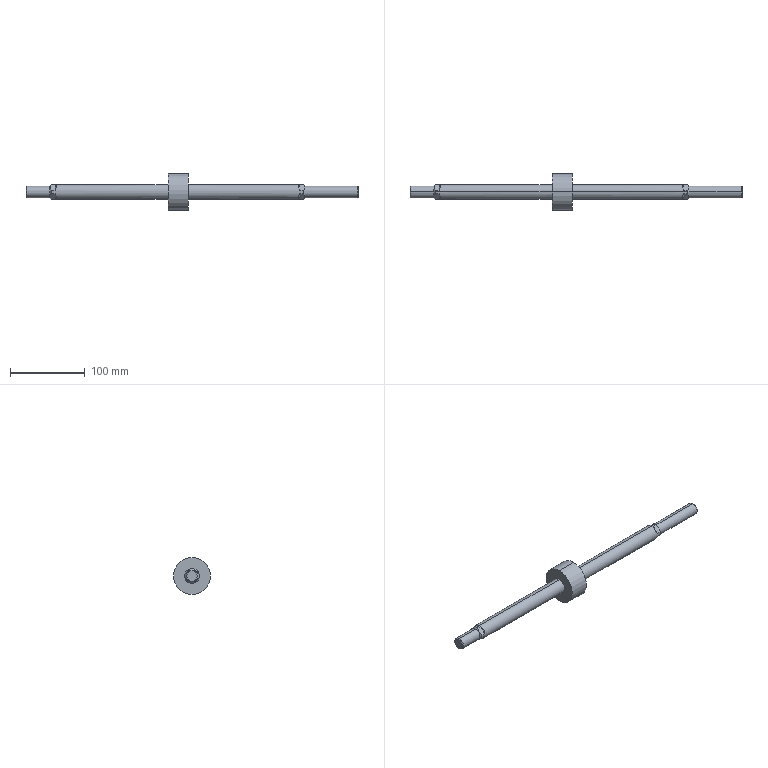Part | SolidWorks | features RefAxis 15, 3DProfileFeature 5, ICE 4, Revolution 2 | 1 solid | 38 faces | box 444 x 49.5 x 49.5 mm | volume 170493 mm3 | plane 20 | cylinder 10 | cone 8 | commonest cylinder face diameters 16 x4 20 x4 49.5 x2
STEP:
#1=CARTESIAN_POINT('',(387.,0.,6.773));
#2=VERTEX_POINT('',#1);
#3=CARTESIAN_POINT('',(387.,0.,-6.773));
#4=VERTEX_POINT('',#3);
#5=CARTESIAN_POINT('',(387.,0.,0.));
#6=DIRECTION('',(-1.,0.,0.));
#7=DIRECTION('',(0.,0.,1.));
#8=AXIS2_PLACEMENT_3D('',#5,#6,#7);
#9=CIRCLE('',#8,6.773);
#10=EDGE_CURVE('',#2,#4,#9,.T.);
#11=ORIENTED_EDGE('',*,*,#10,.T.);
#12=CARTESIAN_POINT('',(385.773,0.,-8.));
#13=VERTEX_POINT('',#12);
#14=CARTESIAN_POINT('',(387.,0.,-6.773));
#15=DIRECTION('',(-0.7071,0.,-0.7071));
#16=VECTOR('',#15,1000.);
#17=LINE('',#14,#16);
#18=EDGE_CURVE('',#4,#13,#17,.T.);
#19=ORIENTED_EDGE('',*,*,#18,.T.);
#20=CARTESIAN_POINT('',(385.773,0.,8.));
#21=VERTEX_POINT('',#20);
#22=CARTESIAN_POINT('',(385.773,0.,0.));
#23=DIRECTION('',(-1.,0.,0.));
#24=DIRECTION('',(0.,0.,1.));
#25=AXIS2_PLACEMENT_3D('',#22,#23,#24);
#26=CIRCLE('',#25,8.);
#27=EDGE_CURVE('',#21,#13,#26,.T.);
#28=ORIENTED_EDGE('',*,*,#27,.F.);
#29=CARTESIAN_POINT('',(387.,0.,6.773));
#30=DIRECTION('',(-0.7071,0.,0.7071));
#31=VECTOR('',#30,1000.);
#32=LINE('',#29,#31);
#33=EDGE_CURVE('',#2,#21,#32,.T.);
#34=ORIENTED_EDGE('',*,*,#33,.F.);
#35=EDGE_LOOP('',(#11,#19,#28,#34));
#36=FACE_OUTER_BOUND('',#35,.T.);
#37=CARTESIAN_POINT('',(387.,0.,0.));
#38=DIRECTION('',(-1.,0.,0.));
#39=DIRECTION('',(0.,0.,1.));
#40=AXIS2_PLACEMENT_3D('',#37,#38,#39);
#41=CONICAL_SURFACE('',#40,6.773,0.7854);
#42=ADVANCED_FACE('',(#36),#41,.T.);
#43=ORIENTED_EDGE('',*,*,#27,.T.);
#44=CARTESIAN_POINT('',(316.,0.,-8.));
#45=VERTEX_POINT('',#44);
#46=CARTESIAN_POINT('',(387.,0.,-8.));
#47=DIRECTION('',(-1.,0.,0.));
#48=VECTOR('',#47,1000.);
#49=LINE('',#46,#48);
#50=EDGE_CURVE('',#13,#45,#49,.T.);
#51=ORIENTED_EDGE('',*,*,#50,.T.);
#52=CARTESIAN_POINT('',(316.,0.,8.));
#53=VERTEX_POINT('',#52);
#54=CARTESIAN_POINT('',(316.,0.,0.));
#55=DIRECTION('',(-1.,0.,0.));
#56=DIRECTION('',(0.,0.,1.));
#57=AXIS2_PLACEMENT_3D('',#54,#55,#56);
#58=CIRCLE('',#57,8.);
#59=EDGE_CURVE('',#53,#45,#58,.T.);
#60=ORIENTED_EDGE('',*,*,#59,.F.);
#61=CARTESIAN_POINT('',(387.,0.,8.));
#62=DIRECTION('',(-1.,0.,0.));
#63=VECTOR('',#62,1000.);
#64=LINE('',#61,#63);
#65=EDGE_CURVE('',#21,#53,#64,.T.);
#66=ORIENTED_EDGE('',*,*,#65,.F.);
#67=EDGE_LOOP('',(#43,#51,#60,#66));
#68=FACE_OUTER_BOUND('',#67,.T.);
#69=CARTESIAN_POINT('',(387.,0.,0.));
#70=DIRECTION('',(-1.,0.,0.));
#71=DIRECTION('',(0.,0.,1.));
#72=AXIS2_PLACEMENT_3D('',#69,#70,#71);
#73=CYLINDRICAL_SURFACE('',#72,8.);
#74=ADVANCED_FACE('',(#68),#73,.T.);
#75=ORIENTED_EDGE('',*,*,#59,.T.);
#76=CARTESIAN_POINT('',(314.,0.,-10.));
#77=VERTEX_POINT('',#76);
#78=CARTESIAN_POINT('',(316.,0.,-8.));
#79=DIRECTION('',(-0.7071,0.,-0.7071));
#80=VECTOR('',#79,1000.);
#81=LINE('',#78,#80);
#82=EDGE_CURVE('',#45,#77,#81,.T.);
#83=ORIENTED_EDGE('',*,*,#82,.T.);
#84=CARTESIAN_POINT('',(314.,2.285,-9.735));
#85=VERTEX_POINT('',#84);
#86=CARTESIAN_POINT('',(314.,0.,0.));
#87=DIRECTION('',(-1.,0.,0.));
#88=DIRECTION('',(0.,0.,1.));
#89=AXIS2_PLACEMENT_3D('',#86,#87,#88);
#90=CIRCLE('',#89,10.);
#91=EDGE_CURVE('',#85,#77,#90,.T.);
#92=ORIENTED_EDGE('',*,*,#91,.F.);
#93=CARTESIAN_POINT('',(314.,9.735,-2.285));
#94=VERTEX_POINT('',#93);
#95=CARTESIAN_POINT('',(314.,2.285,-9.735));
#96=CARTESIAN_POINT('',(314.432,2.865,-9.156));
#97=CARTESIAN_POINT('',(314.804,3.46,-8.561));
#98=CARTESIAN_POINT('',(315.207,4.392,-7.629));
#99=CARTESIAN_POINT('',(315.315,4.711,-7.31));
#100=CARTESIAN_POINT('',(315.462,5.361,-6.66));
#101=CARTESIAN_POINT('',(315.5,5.685,-6.336));
#102=CARTESIAN_POINT('',(315.5,6.335,-5.686));
#103=CARTESIAN_POINT('',(315.463,6.659,-5.362));
#104=CARTESIAN_POINT('',(315.316,7.308,-4.713));
#105=CARTESIAN_POINT('',(315.208,7.628,-4.393));
#106=CARTESIAN_POINT('',(314.805,8.561,-3.46));
#107=CARTESIAN_POINT('',(314.432,9.156,-2.865));
#108=CARTESIAN_POINT('',(314.,9.735,-2.285));
#109=B_SPLINE_CURVE_WITH_KNOTS('',3,(#95,#96,#97,#98,#99,#100,#101,#102,#103,#104,#105,#106,#107,#108),.UNSPECIFIED.,.F.,.F.,(4,2,2,2,2,2,4),(0.000000425,0.002754,0.004131,0.005507,0.006884,0.008261,0.01101),.UNSPECIFIED.);
#110=EDGE_CURVE('',#85,#94,#109,.T.);
#111=ORIENTED_EDGE('',*,*,#110,.T.);
#112=CARTESIAN_POINT('',(314.,9.735,2.285));
#113=VERTEX_POINT('',#112);
#114=CARTESIAN_POINT('',(314.,0.,0.));
#115=DIRECTION('',(-1.,0.,0.));
#116=DIRECTION('',(0.,0.,1.));
#117=AXIS2_PLACEMENT_3D('',#114,#115,#116);
#118=CIRCLE('',#117,10.);
#119=EDGE_CURVE('',#113,#94,#118,.T.);
#120=ORIENTED_EDGE('',*,*,#119,.F.);
#121=CARTESIAN_POINT('',(314.,2.285,9.735));
#122=VERTEX_POINT('',#121);
#123=CARTESIAN_POINT('',(314.,9.735,2.285));
#124=CARTESIAN_POINT('',(314.432,9.156,2.865));
#125=CARTESIAN_POINT('',(314.804,8.561,3.46));
#126=CARTESIAN_POINT('',(315.207,7.629,4.392));
#127=CARTESIAN_POINT('',(315.315,7.31,4.711));
#128=CARTESIAN_POINT('',(315.462,6.66,5.361));
#129=CARTESIAN_POINT('',(315.5,6.336,5.685));
#130=CARTESIAN_POINT('',(315.5,5.686,6.335));
#131=CARTESIAN_POINT('',(315.463,5.362,6.659));
#132=CARTESIAN_POINT('',(315.316,4.713,7.308));
#133=CARTESIAN_POINT('',(315.208,4.393,7.628));
#134=CARTESIAN_POINT('',(314.805,3.46,8.561));
#135=CARTESIAN_POINT('',(314.432,2.865,9.156));
#136=CARTESIAN_POINT('',(314.,2.285,9.735));
#137=B_SPLINE_CURVE_WITH_KNOTS('',3,(#123,#124,#125,#126,#127,#128,#129,#130,#131,#132,#133,#134,#135,#136),.UNSPECIFIED.,.F.,.F.,(4,2,2,2,2,2,4),(0.000000425,0.002754,0.004131,0.005507,0.006884,0.008261,0.01101),.UNSPECIFIED.);
#138=EDGE_CURVE('',#113,#122,#137,.T.);
#139=ORIENTED_EDGE('',*,*,#138,.T.);
#140=CARTESIAN_POINT('',(314.,0.,10.));
#141=VERTEX_POINT('',#140);
#142=CARTESIAN_POINT('',(314.,0.,0.));
#143=DIRECTION('',(-1.,0.,0.));
#144=DIRECTION('',(0.,0.,1.));
#145=AXIS2_PLACEMENT_3D('',#142,#143,#144);
#146=CIRCLE('',#145,10.);
#147=EDGE_CURVE('',#141,#122,#146,.T.);
#148=ORIENTED_EDGE('',*,*,#147,.F.);
#149=CARTESIAN_POINT('',(316.,0.,8.));
#150=DIRECTION('',(-0.7071,0.,0.7071));
#151=VECTOR('',#150,1000.);
#152=LINE('',#149,#151);
#153=EDGE_CURVE('',#53,#141,#152,.T.);
#154=ORIENTED_EDGE('',*,*,#153,.F.);
#155=EDGE_LOOP('',(#75,#83,#92,#111,#120,#139,#148,#154));
#156=FACE_OUTER_BOUND('',#155,.T.);
#157=CARTESIAN_POINT('',(316.,0.,0.));
#158=DIRECTION('',(-1.,0.,0.));
#159=DIRECTION('',(0.,0.,1.));
#160=AXIS2_PLACEMENT_3D('',#157,#158,#159);
#161=CONICAL_SURFACE('',#160,8.,0.7854);
#162=ADVANCED_FACE('',(#156),#161,.T.);
#163=ORIENTED_EDGE('',*,*,#91,.T.);
#164=CARTESIAN_POINT('',(160.,0.,-10.));
#165=VERTEX_POINT('',#164);
#166=CARTESIAN_POINT('',(387.,0.,-10.));
#167=DIRECTION('',(-1.,0.,0.));
#168=VECTOR('',#167,1000.);
#169=LINE('',#166,#168);
#170=EDGE_CURVE('',#77,#165,#169,.T.);
#171=ORIENTED_EDGE('',*,*,#170,.T.);
#172=CARTESIAN_POINT('',(160.,0.,10.));
#173=VERTEX_POINT('',#172);
#174=CARTESIAN_POINT('',(160.,0.,0.));
#175=DIRECTION('',(1.,0.,0.));
#176=DIRECTION('',(0.,0.,1.));
#177=AXIS2_PLACEMENT_3D('',#174,#175,#176);
#178=CIRCLE('',#177,10.);
#179=EDGE_CURVE('',#165,#173,#178,.T.);
#180=ORIENTED_EDGE('',*,*,#179,.T.);
#181=CARTESIAN_POINT('',(387.,0.,10.));
#182=DIRECTION('',(-1.,0.,0.));
#183=VECTOR('',#182,1000.);
#184=LINE('',#181,#183);
#185=EDGE_CURVE('',#141,#173,#184,.T.);
#186=ORIENTED_EDGE('',*,*,#185,.F.);
#187=ORIENTED_EDGE('',*,*,#147,.T.);
#188=CARTESIAN_POINT('',(309.,2.285,9.735));
#189=VERTEX_POINT('',#188);
#190=CARTESIAN_POINT('',(387.,2.285,9.735));
#191=DIRECTION('',(-1.,0.,0.));
#192=VECTOR('',#191,1000.);
#193=LINE('',#190,#192);
#194=EDGE_CURVE('',#122,#189,#193,.T.);
#195=ORIENTED_EDGE('',*,*,#194,.T.);
#196=CARTESIAN_POINT('',(309.,9.735,2.285));
#197=VERTEX_POINT('',#196);
#198=CARTESIAN_POINT('',(309.,2.285,9.735));
#199=CARTESIAN_POINT('',(306.944,6.084,8.844));
#200=CARTESIAN_POINT('',(306.944,8.844,6.084));
#201=CARTESIAN_POINT('',(309.,9.735,2.285));
#202=(BOUNDED_CURVE()B_SPLINE_CURVE(3,(#198,#199,#200,#201),.UNSPECIFIED.,.F.,.T.)B_SPLINE_CURVE_WITH_KNOTS((4,4),(5.728,6.838),.UNSPECIFIED.)CURVE()GEOMETRIC_REPRESENTATION_ITEM()RATIONAL_B_SPLINE_CURVE((1.,0.9,0.9,1.))REPRESENTATION_ITEM(''));
#203=EDGE_CURVE('',#189,#197,#202,.T.);
#204=ORIENTED_EDGE('',*,*,#203,.T.);
#205=CARTESIAN_POINT('',(387.,9.735,2.285));
#206=DIRECTION('',(1.,0.,0.));
#207=VECTOR('',#206,1000.);
#208=LINE('',#205,#207);
#209=EDGE_CURVE('',#197,#113,#208,.T.);
#210=ORIENTED_EDGE('',*,*,#209,.T.);
#211=ORIENTED_EDGE('',*,*,#119,.T.);
#212=CARTESIAN_POINT('',(309.,9.735,-2.285));
#213=VERTEX_POINT('',#212);
#214=CARTESIAN_POINT('',(387.,9.735,-2.285));
#215=DIRECTION('',(-1.,0.,0.));
#216=VECTOR('',#215,1000.);
#217=LINE('',#214,#216);
#218=EDGE_CURVE('',#94,#213,#217,.T.);
#219=ORIENTED_EDGE('',*,*,#218,.T.);
#220=CARTESIAN_POINT('',(309.,2.285,-9.735));
#221=VERTEX_POINT('',#220);
#222=CARTESIAN_POINT('',(309.,9.735,-2.285));
#223=CARTESIAN_POINT('',(306.944,8.844,-6.084));
#224=CARTESIAN_POINT('',(306.944,6.084,-8.844));
#225=CARTESIAN_POINT('',(309.,2.285,-9.735));
#226=(BOUNDED_CURVE()B_SPLINE_CURVE(3,(#222,#223,#224,#225),.UNSPECIFIED.,.F.,.F.)B_SPLINE_CURVE_WITH_KNOTS((4,4),(5.728,6.838),.UNSPECIFIED.)CURVE()GEOMETRIC_REPRESENTATION_ITEM()RATIONAL_B_SPLINE_CURVE((1.,0.9,0.9,1.))REPRESENTATION_ITEM(''));
#227=EDGE_CURVE('',#213,#221,#226,.T.);
#228=ORIENTED_EDGE('',*,*,#227,.T.);
#229=CARTESIAN_POINT('',(387.,2.285,-9.735));
#230=DIRECTION('',(1.,0.,0.));
#231=VECTOR('',#230,1000.);
#232=LINE('',#229,#231);
#233=EDGE_CURVE('',#221,#85,#232,.T.);
#234=ORIENTED_EDGE('',*,*,#233,.T.);
#235=EDGE_LOOP('',(#163,#171,#180,#186,#187,#195,#204,#210,#211,#219,#228,#234));
#236=FACE_OUTER_BOUND('',#235,.T.);
#237=CARTESIAN_POINT('',(387.,0.,0.));
#238=DIRECTION('',(-1.,0.,0.));
#239=DIRECTION('',(0.,0.,1.));
#240=AXIS2_PLACEMENT_3D('',#237,#238,#239);
#241=CYLINDRICAL_SURFACE('',#240,10.);
#242=ADVANCED_FACE('',(#236),#241,.T.);
#243=CARTESIAN_POINT('',(160.,0.,24.75));
#244=VERTEX_POINT('',#243);
#245=CARTESIAN_POINT('',(160.,0.,-24.75));
#246=VERTEX_POINT('',#245);
#247=CARTESIAN_POINT('',(160.,0.,0.));
#248=DIRECTION('',(-1.,0.,0.));
#249=DIRECTION('',(0.,0.,1.));
#250=AXIS2_PLACEMENT_3D('',#247,#248,#249);
#251=CIRCLE('',#250,24.75);
#252=EDGE_CURVE('',#244,#246,#251,.T.);
#253=ORIENTED_EDGE('',*,*,#252,.T.);
#254=CARTESIAN_POINT('',(133.,0.,-24.75));
#255=VERTEX_POINT('',#254);
#256=CARTESIAN_POINT('',(160.,0.,-24.75));
#257=DIRECTION('',(-1.,0.,0.));
#258=VECTOR('',#257,1000.);
#259=LINE('',#256,#258);
#260=EDGE_CURVE('',#246,#255,#259,.T.);
#261=ORIENTED_EDGE('',*,*,#260,.T.);
#262=CARTESIAN_POINT('',(133.,0.,24.75));
#263=VERTEX_POINT('',#262);
#264=CARTESIAN_POINT('',(133.,0.,0.));
#265=DIRECTION('',(-1.,0.,0.));
#266=DIRECTION('',(0.,0.,1.));
#267=AXIS2_PLACEMENT_3D('',#264,#265,#266);
#268=CIRCLE('',#267,24.75);
#269=EDGE_CURVE('',#263,#255,#268,.T.);
#270=ORIENTED_EDGE('',*,*,#269,.F.);
#271=CARTESIAN_POINT('',(160.,0.,24.75));
#272=DIRECTION('',(-1.,0.,0.));
#273=VECTOR('',#272,1000.);
#274=LINE('',#271,#273);
#275=EDGE_CURVE('',#244,#263,#274,.T.);
#276=ORIENTED_EDGE('',*,*,#275,.F.);
#277=EDGE_LOOP('',(#253,#261,#270,#276));
#278=FACE_OUTER_BOUND('',#277,.T.);
#279=CARTESIAN_POINT('',(160.,0.,0.));
#280=DIRECTION('',(-1.,0.,0.));
#281=DIRECTION('',(0.,0.,1.));
#282=AXIS2_PLACEMENT_3D('',#279,#280,#281);
#283=CYLINDRICAL_SURFACE('',#282,24.75);
#284=ADVANCED_FACE('',(#278),#283,.T.);
#285=CARTESIAN_POINT('',(133.,0.,10.));
#286=VERTEX_POINT('',#285);
#287=CARTESIAN_POINT('',(133.,0.,-10.));
#288=VERTEX_POINT('',#287);
#289=CARTESIAN_POINT('',(133.,0.,0.));
#290=DIRECTION('',(-1.,0.,0.));
#291=DIRECTION('',(0.,0.,1.));
#292=AXIS2_PLACEMENT_3D('',#289,#290,#291);
#293=CIRCLE('',#292,10.);
#294=EDGE_CURVE('',#286,#288,#293,.T.);
#295=ORIENTED_EDGE('',*,*,#294,.T.);
#296=CARTESIAN_POINT('',(-23.,0.,-10.));
#297=VERTEX_POINT('',#296);
#298=CARTESIAN_POINT('',(160.,0.,-10.));
#299=DIRECTION('',(-1.,0.,0.));
#300=VECTOR('',#299,1000.);
#301=LINE('',#298,#300);
#302=EDGE_CURVE('',#288,#297,#301,.T.);
#303=ORIENTED_EDGE('',*,*,#302,.T.);
#304=CARTESIAN_POINT('',(-23.,2.285,-9.735));
#305=VERTEX_POINT('',#304);
#306=CARTESIAN_POINT('',(-23.,0.,0.));
#307=DIRECTION('',(-1.,0.,0.));
#308=DIRECTION('',(0.,0.,1.));
#309=AXIS2_PLACEMENT_3D('',#306,#307,#308);
#310=CIRCLE('',#309,10.);
#311=EDGE_CURVE('',#305,#297,#310,.T.);
#312=ORIENTED_EDGE('',*,*,#311,.F.);
#313=CARTESIAN_POINT('',(-18.,2.285,-9.735));
#314=VERTEX_POINT('',#313);
#315=CARTESIAN_POINT('',(160.,2.285,-9.735));
#316=DIRECTION('',(1.,0.,0.));
#317=VECTOR('',#316,1000.);
#318=LINE('',#315,#317);
#319=EDGE_CURVE('',#305,#314,#318,.T.);
#320=ORIENTED_EDGE('',*,*,#319,.T.);
#321=CARTESIAN_POINT('',(-18.,9.735,-2.285));
#322=VERTEX_POINT('',#321);
#323=CARTESIAN_POINT('',(-18.,2.285,-9.735));
#324=CARTESIAN_POINT('',(-15.944,6.084,-8.844));
#325=CARTESIAN_POINT('',(-15.944,8.844,-6.084));
#326=CARTESIAN_POINT('',(-18.,9.735,-2.285));
#327=(BOUNDED_CURVE()B_SPLINE_CURVE(3,(#323,#324,#325,#326),.UNSPECIFIED.,.F.,.F.)B_SPLINE_CURVE_WITH_KNOTS((4,4),(2.587,3.696),.UNSPECIFIED.)CURVE()GEOMETRIC_REPRESENTATION_ITEM()RATIONAL_B_SPLINE_CURVE((1.,0.9,0.9,1.))REPRESENTATION_ITEM(''));
#328=EDGE_CURVE('',#314,#322,#327,.T.);
#329=ORIENTED_EDGE('',*,*,#328,.T.);
#330=CARTESIAN_POINT('',(-23.,9.735,-2.285));
#331=VERTEX_POINT('',#330);
#332=CARTESIAN_POINT('',(160.,9.735,-2.285));
#333=DIRECTION('',(-1.,0.,0.));
#334=VECTOR('',#333,1000.);
#335=LINE('',#332,#334);
#336=EDGE_CURVE('',#322,#331,#335,.T.);
#337=ORIENTED_EDGE('',*,*,#336,.T.);
#338=CARTESIAN_POINT('',(-23.,9.735,2.285));
#339=VERTEX_POINT('',#338);
#340=CARTESIAN_POINT('',(-23.,0.,0.));
#341=DIRECTION('',(-1.,0.,0.));
#342=DIRECTION('',(0.,0.,1.));
#343=AXIS2_PLACEMENT_3D('',#340,#341,#342);
#344=CIRCLE('',#343,10.);
#345=EDGE_CURVE('',#339,#331,#344,.T.);
#346=ORIENTED_EDGE('',*,*,#345,.F.);
#347=CARTESIAN_POINT('',(-18.,9.735,2.285));
#348=VERTEX_POINT('',#347);
#349=CARTESIAN_POINT('',(160.,9.735,2.285));
#350=DIRECTION('',(1.,0.,0.));
#351=VECTOR('',#350,1000.);
#352=LINE('',#349,#351);
#353=EDGE_CURVE('',#339,#348,#352,.T.);
#354=ORIENTED_EDGE('',*,*,#353,.T.);
#355=CARTESIAN_POINT('',(-18.,2.285,9.735));
#356=VERTEX_POINT('',#355);
#357=CARTESIAN_POINT('',(-18.,9.735,2.285));
#358=CARTESIAN_POINT('',(-15.944,8.844,6.084));
#359=CARTESIAN_POINT('',(-15.944,6.084,8.844));
#360=CARTESIAN_POINT('',(-18.,2.285,9.735));
#361=(BOUNDED_CURVE()B_SPLINE_CURVE(3,(#357,#358,#359,#360),.UNSPECIFIED.,.F.,.F.)B_SPLINE_CURVE_WITH_KNOTS((4,4),(2.587,3.696),.UNSPECIFIED.)CURVE()GEOMETRIC_REPRESENTATION_ITEM()RATIONAL_B_SPLINE_CURVE((1.,0.9,0.9,1.))REPRESENTATION_ITEM(''));
#362=EDGE_CURVE('',#348,#356,#361,.T.);
#363=ORIENTED_EDGE('',*,*,#362,.T.);
#364=CARTESIAN_POINT('',(-23.,2.285,9.735));
#365=VERTEX_POINT('',#364);
#366=CARTESIAN_POINT('',(160.,2.285,9.735));
#367=DIRECTION('',(-1.,0.,0.));
#368=VECTOR('',#367,1000.);
#369=LINE('',#366,#368);
#370=EDGE_CURVE('',#356,#365,#369,.T.);
#371=ORIENTED_EDGE('',*,*,#370,.T.);
#372=CARTESIAN_POINT('',(-23.,0.,10.));
#373=VERTEX_POINT('',#372);
#374=CARTESIAN_POINT('',(-23.,0.,0.));
#375=DIRECTION('',(-1.,0.,0.));
#376=DIRECTION('',(0.,0.,1.));
#377=AXIS2_PLACEMENT_3D('',#374,#375,#376);
#378=CIRCLE('',#377,10.);
#379=EDGE_CURVE('',#373,#365,#378,.T.);
#380=ORIENTED_EDGE('',*,*,#379,.F.);
#381=CARTESIAN_POINT('',(160.,0.,10.));
#382=DIRECTION('',(-1.,0.,0.));
#383=VECTOR('',#382,1000.);
#384=LINE('',#381,#383);
#385=EDGE_CURVE('',#286,#373,#384,.T.);
#386=ORIENTED_EDGE('',*,*,#385,.F.);
#387=EDGE_LOOP('',(#295,#303,#312,#320,#329,#337,#346,#354,#363,#371,#380,#386));
#388=FACE_OUTER_BOUND('',#387,.T.);
#389=CARTESIAN_POINT('',(160.,0.,0.));
#390=DIRECTION('',(-1.,0.,0.));
#391=DIRECTION('',(0.,0.,1.));
#392=AXIS2_PLACEMENT_3D('',#389,#390,#391);
#393=CYLINDRICAL_SURFACE('',#392,10.);
#394=ADVANCED_FACE('',(#388),#393,.T.);
#395=CARTESIAN_POINT('',(-25.,0.,8.));
#396=VERTEX_POINT('',#395);
#397=CARTESIAN_POINT('',(-25.,0.,-8.));
#398=VERTEX_POINT('',#397);
#399=CARTESIAN_POINT('',(-25.,0.,0.));
#400=DIRECTION('',(-1.,0.,0.));
#401=DIRECTION('',(0.,0.,1.));
#402=AXIS2_PLACEMENT_3D('',#399,#400,#401);
#403=CIRCLE('',#402,8.);
#404=EDGE_CURVE('',#396,#398,#403,.T.);
#405=ORIENTED_EDGE('',*,*,#404,.F.);
#406=CARTESIAN_POINT('',(-23.,0.,10.));
#407=DIRECTION('',(0.7071,0.,0.7071));
#408=VECTOR('',#407,1000.);
#409=LINE('',#406,#408);
#410=EDGE_CURVE('',#396,#373,#409,.T.);
#411=ORIENTED_EDGE('',*,*,#410,.T.);
#412=ORIENTED_EDGE('',*,*,#379,.T.);
#413=CARTESIAN_POINT('',(-23.,2.285,9.735));
#414=CARTESIAN_POINT('',(-23.432,2.865,9.156));
#415=CARTESIAN_POINT('',(-23.804,3.46,8.561));
#416=CARTESIAN_POINT('',(-24.207,4.392,7.629));
#417=CARTESIAN_POINT('',(-24.315,4.711,7.31));
#418=CARTESIAN_POINT('',(-24.462,5.361,6.66));
#419=CARTESIAN_POINT('',(-24.5,5.685,6.336));
#420=CARTESIAN_POINT('',(-24.5,6.335,5.686));
#421=CARTESIAN_POINT('',(-24.463,6.659,5.362));
#422=CARTESIAN_POINT('',(-24.316,7.308,4.713));
#423=CARTESIAN_POINT('',(-24.208,7.628,4.393));
#424=CARTESIAN_POINT('',(-23.805,8.561,3.46));
#425=CARTESIAN_POINT('',(-23.432,9.156,2.865));
#426=CARTESIAN_POINT('',(-23.,9.735,2.285));
#427=B_SPLINE_CURVE_WITH_KNOTS('',3,(#413,#414,#415,#416,#417,#418,#419,#420,#421,#422,#423,#424,#425,#426),.UNSPECIFIED.,.F.,.F.,(4,2,2,2,2,2,4),(0.000000425,0.002754,0.004131,0.005507,0.006884,0.008261,0.01101),.UNSPECIFIED.);
#428=EDGE_CURVE('',#365,#339,#427,.T.);
#429=ORIENTED_EDGE('',*,*,#428,.T.);
#430=ORIENTED_EDGE('',*,*,#345,.T.);
#431=CARTESIAN_POINT('',(-23.,9.735,-2.285));
#432=CARTESIAN_POINT('',(-23.432,9.156,-2.865));
#433=CARTESIAN_POINT('',(-23.804,8.561,-3.46));
#434=CARTESIAN_POINT('',(-24.207,7.629,-4.392));
#435=CARTESIAN_POINT('',(-24.315,7.31,-4.711));
#436=CARTESIAN_POINT('',(-24.462,6.66,-5.361));
#437=CARTESIAN_POINT('',(-24.5,6.336,-5.685));
#438=CARTESIAN_POINT('',(-24.5,5.686,-6.335));
#439=CARTESIAN_POINT('',(-24.463,5.362,-6.659));
#440=CARTESIAN_POINT('',(-24.316,4.713,-7.308));
#441=CARTESIAN_POINT('',(-24.208,4.393,-7.628));
#442=CARTESIAN_POINT('',(-23.805,3.46,-8.561));
#443=CARTESIAN_POINT('',(-23.432,2.865,-9.156));
#444=CARTESIAN_POINT('',(-23.,2.285,-9.735));
#445=B_SPLINE_CURVE_WITH_KNOTS('',3,(#431,#432,#433,#434,#435,#436,#437,#438,#439,#440,#441,#442,#443,#444),.UNSPECIFIED.,.F.,.F.,(4,2,2,2,2,2,4),(0.000000425,0.002754,0.004131,0.005507,0.006884,0.008261,0.01101),.UNSPECIFIED.);
#446=EDGE_CURVE('',#331,#305,#445,.T.);
#447=ORIENTED_EDGE('',*,*,#446,.T.);
#448=ORIENTED_EDGE('',*,*,#311,.T.);
#449=CARTESIAN_POINT('',(-23.,0.,-10.));
#450=DIRECTION('',(0.7071,0.,-0.7071));
#451=VECTOR('',#450,1000.);
#452=LINE('',#449,#451);
#453=EDGE_CURVE('',#398,#297,#452,.T.);
#454=ORIENTED_EDGE('',*,*,#453,.F.);
#455=EDGE_LOOP('',(#405,#411,#412,#429,#430,#447,#448,#454));
#456=FACE_OUTER_BOUND('',#455,.T.);
#457=CARTESIAN_POINT('',(-23.,0.,0.));
#458=DIRECTION('',(1.,0.,0.));
#459=DIRECTION('',(0.,0.,-1.));
#460=AXIS2_PLACEMENT_3D('',#457,#458,#459);
#461=CONICAL_SURFACE('',#460,10.,0.7854);
#462=ADVANCED_FACE('',(#456),#461,.T.);
#463=ORIENTED_EDGE('',*,*,#404,.T.);
#464=CARTESIAN_POINT('',(-56.08,0.,-8.));
#465=VERTEX_POINT('',#464);
#466=CARTESIAN_POINT('',(160.,0.,-8.));
#467=DIRECTION('',(-1.,0.,0.));
#468=VECTOR('',#467,1000.);
#469=LINE('',#466,#468);
#470=EDGE_CURVE('',#398,#465,#469,.T.);
#471=ORIENTED_EDGE('',*,*,#470,.T.);
#472=CARTESIAN_POINT('',(-56.08,0.,8.));
#473=VERTEX_POINT('',#472);
#474=CARTESIAN_POINT('',(-56.08,0.,0.));
#475=DIRECTION('',(-1.,0.,0.));
#476=DIRECTION('',(0.,0.,1.));
#477=AXIS2_PLACEMENT_3D('',#474,#475,#476);
#478=CIRCLE('',#477,8.);
#479=EDGE_CURVE('',#473,#465,#478,.T.);
#480=ORIENTED_EDGE('',*,*,#479,.F.);
#481=CARTESIAN_POINT('',(160.,0.,8.));
#482=DIRECTION('',(-1.,0.,0.));
#483=VECTOR('',#482,1000.);
#484=LINE('',#481,#483);
#485=EDGE_CURVE('',#396,#473,#484,.T.);
#486=ORIENTED_EDGE('',*,*,#485,.F.);
#487=EDGE_LOOP('',(#463,#471,#480,#486));
#488=FACE_OUTER_BOUND('',#487,.T.);
#489=CARTESIAN_POINT('',(160.,0.,0.));
#490=DIRECTION('',(-1.,0.,0.));
#491=DIRECTION('',(0.,0.,1.));
#492=AXIS2_PLACEMENT_3D('',#489,#490,#491);
#493=CYLINDRICAL_SURFACE('',#492,8.);
#494=ADVANCED_FACE('',(#488),#493,.T.);
#495=CARTESIAN_POINT('',(-57.,0.,7.08));
#496=VERTEX_POINT('',#495);
#497=CARTESIAN_POINT('',(-57.,0.,-7.08));
#498=VERTEX_POINT('',#497);
#499=CARTESIAN_POINT('',(-57.,0.,0.));
#500=DIRECTION('',(-1.,0.,0.));
#501=DIRECTION('',(0.,0.,1.));
#502=AXIS2_PLACEMENT_3D('',#499,#500,#501);
#503=CIRCLE('',#502,7.08);
#504=EDGE_CURVE('',#496,#498,#503,.T.);
#505=ORIENTED_EDGE('',*,*,#504,.F.);
#506=CARTESIAN_POINT('',(-56.08,0.,8.));
#507=DIRECTION('',(0.7071,0.,0.7071));
#508=VECTOR('',#507,1000.);
#509=LINE('',#506,#508);
#510=EDGE_CURVE('',#496,#473,#509,.T.);
#511=ORIENTED_EDGE('',*,*,#510,.T.);
#512=ORIENTED_EDGE('',*,*,#479,.T.);
#513=CARTESIAN_POINT('',(-56.08,0.,-8.));
#514=DIRECTION('',(0.7071,0.,-0.7071));
#515=VECTOR('',#514,1000.);
#516=LINE('',#513,#515);
#517=EDGE_CURVE('',#498,#465,#516,.T.);
#518=ORIENTED_EDGE('',*,*,#517,.F.);
#519=EDGE_LOOP('',(#505,#511,#512,#518));
#520=FACE_OUTER_BOUND('',#519,.T.);
#521=CARTESIAN_POINT('',(-56.08,0.,0.));
#522=DIRECTION('',(1.,0.,0.));
#523=DIRECTION('',(0.,0.,-1.));
#524=AXIS2_PLACEMENT_3D('',#521,#522,#523);
#525=CONICAL_SURFACE('',#524,8.,0.7854);
#526=ADVANCED_FACE('',(#520),#525,.T.);
#527=CARTESIAN_POINT('',(-57.,0.,0.));
#528=DIRECTION('',(-1.,0.,0.));
#529=DIRECTION('',(0.,0.,1.));
#530=AXIS2_PLACEMENT_3D('',#527,#528,#529);
#531=CIRCLE('',#530,7.08);
#532=EDGE_CURVE('',#498,#496,#531,.T.);
#533=ORIENTED_EDGE('',*,*,#532,.T.);
#534=ORIENTED_EDGE('',*,*,#504,.T.);
#535=EDGE_LOOP('',(#533,#534));
#536=FACE_OUTER_BOUND('',#535,.T.);
#537=CARTESIAN_POINT('',(-57.,0.,0.));
#538=DIRECTION('',(1.,0.,0.));
#539=DIRECTION('',(0.,0.,-1.));
#540=AXIS2_PLACEMENT_3D('',#537,#538,#539);
#541=PLANE('',#540);
#542=ADVANCED_FACE('',(#536),#541,.F.);
#543=ORIENTED_EDGE('',*,*,#510,.F.);
#544=ORIENTED_EDGE('',*,*,#532,.F.);
#545=ORIENTED_EDGE('',*,*,#517,.T.);
#546=CARTESIAN_POINT('',(-56.08,0.,0.));
#547=DIRECTION('',(-1.,0.,0.));
#548=DIRECTION('',(0.,0.,1.));
#549=AXIS2_PLACEMENT_3D('',#546,#547,#548);
#550=CIRCLE('',#549,8.);
#551=EDGE_CURVE('',#465,#473,#550,.T.);
#552=ORIENTED_EDGE('',*,*,#551,.T.);
#553=EDGE_LOOP('',(#543,#544,#545,#552));
#554=FACE_OUTER_BOUND('',#553,.T.);
#555=CARTESIAN_POINT('',(-56.08,0.,0.));
#556=DIRECTION('',(1.,0.,0.));
#557=DIRECTION('',(0.,0.,-1.));
#558=AXIS2_PLACEMENT_3D('',#555,#556,#557);
#559=CONICAL_SURFACE('',#558,8.,0.7854);
#560=ADVANCED_FACE('',(#554),#559,.T.);
#561=ORIENTED_EDGE('',*,*,#470,.F.);
#562=CARTESIAN_POINT('',(-25.,0.,0.));
#563=DIRECTION('',(-1.,0.,0.));
#564=DIRECTION('',(0.,0.,1.));
#565=AXIS2_PLACEMENT_3D('',#562,#563,#564);
#566=CIRCLE('',#565,8.);
#567=EDGE_CURVE('',#398,#396,#566,.T.);
#568=ORIENTED_EDGE('',*,*,#567,.T.);
#569=ORIENTED_EDGE('',*,*,#485,.T.);
#570=ORIENTED_EDGE('',*,*,#551,.F.);
#571=EDGE_LOOP('',(#561,#568,#569,#570));
#572=FACE_OUTER_BOUND('',#571,.T.);
#573=CARTESIAN_POINT('',(160.,0.,0.));
#574=DIRECTION('',(-1.,0.,0.));
#575=DIRECTION('',(0.,0.,1.));
#576=AXIS2_PLACEMENT_3D('',#573,#574,#575);
#577=CYLINDRICAL_SURFACE('',#576,8.);
#578=ADVANCED_FACE('',(#572),#577,.T.);
#579=ORIENTED_EDGE('',*,*,#410,.F.);
#580=ORIENTED_EDGE('',*,*,#567,.F.);
#581=ORIENTED_EDGE('',*,*,#453,.T.);
#582=CARTESIAN_POINT('',(-23.,-2.285,-9.735));
#583=VERTEX_POINT('',#582);
#584=CARTESIAN_POINT('',(-23.,0.,0.));
#585=DIRECTION('',(-1.,0.,0.));
#586=DIRECTION('',(0.,0.,1.));
#587=AXIS2_PLACEMENT_3D('',#584,#585,#586);
#588=CIRCLE('',#587,10.);
#589=EDGE_CURVE('',#297,#583,#588,.T.);
#590=ORIENTED_EDGE('',*,*,#589,.T.);
#591=CARTESIAN_POINT('',(-23.,-9.735,-2.285));
#592=VERTEX_POINT('',#591);
#593=CARTESIAN_POINT('',(-23.,-2.285,-9.735));
#594=CARTESIAN_POINT('',(-23.432,-2.865,-9.156));
#595=CARTESIAN_POINT('',(-23.804,-3.46,-8.561));
#596=CARTESIAN_POINT('',(-24.207,-4.392,-7.629));
#597=CARTESIAN_POINT('',(-24.315,-4.711,-7.31));
#598=CARTESIAN_POINT('',(-24.462,-5.361,-6.66));
#599=CARTESIAN_POINT('',(-24.5,-5.685,-6.336));
#600=CARTESIAN_POINT('',(-24.5,-6.335,-5.686));
#601=CARTESIAN_POINT('',(-24.463,-6.659,-5.362));
#602=CARTESIAN_POINT('',(-24.316,-7.308,-4.713));
#603=CARTESIAN_POINT('',(-24.208,-7.628,-4.393));
#604=CARTESIAN_POINT('',(-23.805,-8.561,-3.46));
#605=CARTESIAN_POINT('',(-23.432,-9.156,-2.865));
#606=CARTESIAN_POINT('',(-23.,-9.735,-2.285));
#607=B_SPLINE_CURVE_WITH_KNOTS('',3,(#593,#594,#595,#596,#597,#598,#599,#600,#601,#602,#603,#604,#605,#606),.UNSPECIFIED.,.F.,.F.,(4,2,2,2,2,2,4),(0.000000425,0.002754,0.004131,0.005507,0.006884,0.008261,0.01101),.UNSPECIFIED.);
#608=EDGE_CURVE('',#583,#592,#607,.T.);
#609=ORIENTED_EDGE('',*,*,#608,.T.);
#610=CARTESIAN_POINT('',(-23.,-9.735,2.285));
#611=VERTEX_POINT('',#610);
#612=CARTESIAN_POINT('',(-23.,0.,0.));
#613=DIRECTION('',(-1.,0.,0.));
#614=DIRECTION('',(0.,0.,1.));
#615=AXIS2_PLACEMENT_3D('',#612,#613,#614);
#616=CIRCLE('',#615,10.);
#617=EDGE_CURVE('',#592,#611,#616,.T.);
#618=ORIENTED_EDGE('',*,*,#617,.T.);
#619=CARTESIAN_POINT('',(-23.,-2.285,9.735));
#620=VERTEX_POINT('',#619);
#621=CARTESIAN_POINT('',(-23.,-9.735,2.285));
#622=CARTESIAN_POINT('',(-23.432,-9.156,2.865));
#623=CARTESIAN_POINT('',(-23.804,-8.561,3.46));
#624=CARTESIAN_POINT('',(-24.207,-7.629,4.392));
#625=CARTESIAN_POINT('',(-24.315,-7.31,4.711));
#626=CARTESIAN_POINT('',(-24.462,-6.66,5.361));
#627=CARTESIAN_POINT('',(-24.5,-6.336,5.685));
#628=CARTESIAN_POINT('',(-24.5,-5.686,6.335));
#629=CARTESIAN_POINT('',(-24.463,-5.362,6.659));
#630=CARTESIAN_POINT('',(-24.316,-4.713,7.308));
#631=CARTESIAN_POINT('',(-24.208,-4.393,7.628));
#632=CARTESIAN_POINT('',(-23.805,-3.46,8.561));
#633=CARTESIAN_POINT('',(-23.432,-2.865,9.156));
#634=CARTESIAN_POINT('',(-23.,-2.285,9.735));
#635=B_SPLINE_CURVE_WITH_KNOTS('',3,(#621,#622,#623,#624,#625,#626,#627,#628,#629,#630,#631,#632,#633,#634),.UNSPECIFIED.,.F.,.F.,(4,2,2,2,2,2,4),(0.000000425,0.002754,0.004131,0.005507,0.006884,0.008261,0.01101),.UNSPECIFIED.);
#636=EDGE_CURVE('',#611,#620,#635,.T.);
#637=ORIENTED_EDGE('',*,*,#636,.T.);
#638=CARTESIAN_POINT('',(-23.,0.,0.));
#639=DIRECTION('',(-1.,0.,0.));
#640=DIRECTION('',(0.,0.,1.));
#641=AXIS2_PLACEMENT_3D('',#638,#639,#640);
#642=CIRCLE('',#641,10.);
#643=EDGE_CURVE('',#620,#373,#642,.T.);
#644=ORIENTED_EDGE('',*,*,#643,.T.);
#645=EDGE_LOOP('',(#579,#580,#581,#590,#609,#618,#637,#644));
#646=FACE_OUTER_BOUND('',#645,.T.);
#647=CARTESIAN_POINT('',(-23.,0.,0.));
#648=DIRECTION('',(1.,0.,0.));
#649=DIRECTION('',(0.,0.,-1.));
#650=AXIS2_PLACEMENT_3D('',#647,#648,#649);
#651=CONICAL_SURFACE('',#650,10.,0.7854);
#652=ADVANCED_FACE('',(#646),#651,.T.);
#653=ORIENTED_EDGE('',*,*,#302,.F.);
#654=CARTESIAN_POINT('',(133.,0.,0.));
#655=DIRECTION('',(-1.,0.,0.));
#656=DIRECTION('',(0.,0.,1.));
#657=AXIS2_PLACEMENT_3D('',#654,#655,#656);
#658=CIRCLE('',#657,10.);
#659=EDGE_CURVE('',#288,#286,#658,.T.);
#660=ORIENTED_EDGE('',*,*,#659,.T.);
#661=ORIENTED_EDGE('',*,*,#385,.T.);
#662=ORIENTED_EDGE('',*,*,#643,.F.);
#663=CARTESIAN_POINT('',(-18.,-2.285,9.735));
#664=VERTEX_POINT('',#663);
#665=CARTESIAN_POINT('',(160.,-2.285,9.735));
#666=DIRECTION('',(1.,0.,0.));
#667=VECTOR('',#666,1000.);
#668=LINE('',#665,#667);
#669=EDGE_CURVE('',#620,#664,#668,.T.);
#670=ORIENTED_EDGE('',*,*,#669,.T.);
#671=CARTESIAN_POINT('',(-18.,-9.735,2.285));
#672=VERTEX_POINT('',#671);
#673=CARTESIAN_POINT('',(-18.,-2.285,9.735));
#674=CARTESIAN_POINT('',(-15.944,-6.084,8.844));
#675=CARTESIAN_POINT('',(-15.944,-8.844,6.084));
#676=CARTESIAN_POINT('',(-18.,-9.735,2.285));
#677=(BOUNDED_CURVE()B_SPLINE_CURVE(3,(#673,#674,#675,#676),.UNSPECIFIED.,.F.,.F.)B_SPLINE_CURVE_WITH_KNOTS((4,4),(2.587,3.696),.UNSPECIFIED.)CURVE()GEOMETRIC_REPRESENTATION_ITEM()RATIONAL_B_SPLINE_CURVE((1.,0.9,0.9,1.))REPRESENTATION_ITEM(''));
#678=EDGE_CURVE('',#664,#672,#677,.T.);
#679=ORIENTED_EDGE('',*,*,#678,.T.);
#680=CARTESIAN_POINT('',(160.,-9.735,2.285));
#681=DIRECTION('',(-1.,0.,0.));
#682=VECTOR('',#681,1000.);
#683=LINE('',#680,#682);
#684=EDGE_CURVE('',#672,#611,#683,.T.);
#685=ORIENTED_EDGE('',*,*,#684,.T.);
#686=ORIENTED_EDGE('',*,*,#617,.F.);
#687=CARTESIAN_POINT('',(-18.,-9.735,-2.285));
#688=VERTEX_POINT('',#687);
#689=CARTESIAN_POINT('',(160.,-9.735,-2.285));
#690=DIRECTION('',(1.,0.,0.));
#691=VECTOR('',#690,1000.);
#692=LINE('',#689,#691);
#693=EDGE_CURVE('',#592,#688,#692,.T.);
#694=ORIENTED_EDGE('',*,*,#693,.T.);
#695=CARTESIAN_POINT('',(-18.,-2.285,-9.735));
#696=VERTEX_POINT('',#695);
#697=CARTESIAN_POINT('',(-18.,-9.735,-2.285));
#698=CARTESIAN_POINT('',(-15.944,-8.844,-6.084));
#699=CARTESIAN_POINT('',(-15.944,-6.084,-8.844));
#700=CARTESIAN_POINT('',(-18.,-2.285,-9.735));
#701=(BOUNDED_CURVE()B_SPLINE_CURVE(3,(#697,#698,#699,#700),.UNSPECIFIED.,.F.,.T.)B_SPLINE_CURVE_WITH_KNOTS((4,4),(2.587,3.696),.UNSPECIFIED.)CURVE()GEOMETRIC_REPRESENTATION_ITEM()RATIONAL_B_SPLINE_CURVE((1.,0.9,0.9,1.))REPRESENTATION_ITEM(''));
#702=EDGE_CURVE('',#688,#696,#701,.T.);
#703=ORIENTED_EDGE('',*,*,#702,.T.);
#704=CARTESIAN_POINT('',(160.,-2.285,-9.735));
#705=DIRECTION('',(-1.,0.,0.));
#706=VECTOR('',#705,1000.);
#707=LINE('',#704,#706);
#708=EDGE_CURVE('',#696,#583,#707,.T.);
#709=ORIENTED_EDGE('',*,*,#708,.T.);
#710=ORIENTED_EDGE('',*,*,#589,.F.);
#711=EDGE_LOOP('',(#653,#660,#661,#662,#670,#679,#685,#686,#694,#703,#709,#710));
#712=FACE_OUTER_BOUND('',#711,.T.);
#713=CARTESIAN_POINT('',(160.,0.,0.));
#714=DIRECTION('',(-1.,0.,0.));
#715=DIRECTION('',(0.,0.,1.));
#716=AXIS2_PLACEMENT_3D('',#713,#714,#715);
#717=CYLINDRICAL_SURFACE('',#716,10.);
#718=ADVANCED_FACE('',(#712),#717,.T.);
#719=ORIENTED_EDGE('',*,*,#294,.F.);
#720=ORIENTED_EDGE('',*,*,#659,.F.);
#721=EDGE_LOOP('',(#719,#720));
#722=FACE_BOUND('',#721,.T.);
#723=ORIENTED_EDGE('',*,*,#269,.T.);
#724=CARTESIAN_POINT('',(133.,0.,0.));
#725=DIRECTION('',(-1.,0.,0.));
#726=DIRECTION('',(0.,0.,1.));
#727=AXIS2_PLACEMENT_3D('',#724,#725,#726);
#728=CIRCLE('',#727,24.75);
#729=EDGE_CURVE('',#255,#263,#728,.T.);
#730=ORIENTED_EDGE('',*,*,#729,.T.);
#731=EDGE_LOOP('',(#723,#730));
#732=FACE_OUTER_BOUND('',#731,.T.);
#733=CARTESIAN_POINT('',(133.,10.,0.));
#734=DIRECTION('',(1.,0.,0.));
#735=DIRECTION('',(0.,0.,-1.));
#736=AXIS2_PLACEMENT_3D('',#733,#734,#735);
#737=PLANE('',#736);
#738=ADVANCED_FACE('',(#722,#732),#737,.F.);
#739=ORIENTED_EDGE('',*,*,#260,.F.);
#740=CARTESIAN_POINT('',(160.,0.,0.));
#741=DIRECTION('',(-1.,0.,0.));
#742=DIRECTION('',(0.,0.,1.));
#743=AXIS2_PLACEMENT_3D('',#740,#741,#742);
#744=CIRCLE('',#743,24.75);
#745=EDGE_CURVE('',#246,#244,#744,.T.);
#746=ORIENTED_EDGE('',*,*,#745,.T.);
#747=ORIENTED_EDGE('',*,*,#275,.T.);
#748=ORIENTED_EDGE('',*,*,#729,.F.);
#749=EDGE_LOOP('',(#739,#746,#747,#748));
#750=FACE_OUTER_BOUND('',#749,.T.);
#751=CARTESIAN_POINT('',(160.,0.,0.));
#752=DIRECTION('',(-1.,0.,0.));
#753=DIRECTION('',(0.,0.,1.));
#754=AXIS2_PLACEMENT_3D('',#751,#752,#753);
#755=CYLINDRICAL_SURFACE('',#754,24.75);
#756=ADVANCED_FACE('',(#750),#755,.T.);
#757=CARTESIAN_POINT('',(160.,0.,0.));
#758=DIRECTION('',(1.,0.,0.));
#759=DIRECTION('',(0.,0.,1.));
#760=AXIS2_PLACEMENT_3D('',#757,#758,#759);
#761=CIRCLE('',#760,10.);
#762=EDGE_CURVE('',#173,#165,#761,.T.);
#763=ORIENTED_EDGE('',*,*,#762,.F.);
#764=ORIENTED_EDGE('',*,*,#179,.F.);
#765=EDGE_LOOP('',(#763,#764));
#766=FACE_BOUND('',#765,.T.);
#767=ORIENTED_EDGE('',*,*,#252,.F.);
#768=ORIENTED_EDGE('',*,*,#745,.F.);
#769=EDGE_LOOP('',(#767,#768));
#770=FACE_OUTER_BOUND('',#769,.T.);
#771=CARTESIAN_POINT('',(160.,24.75,0.));
#772=DIRECTION('',(-1.,0.,0.));
#773=DIRECTION('',(0.,0.,1.));
#774=AXIS2_PLACEMENT_3D('',#771,#772,#773);
#775=PLANE('',#774);
#776=ADVANCED_FACE('',(#766,#770),#775,.F.);
#777=CARTESIAN_POINT('',(-18.,6.01,-18.031));
#778=DIRECTION('',(0.,-0.7071,0.7071));
#779=VECTOR('',#778,1000.);
#780=LINE('',#777,#779);
#781=EDGE_CURVE('',#696,#688,#780,.T.);
#782=ORIENTED_EDGE('',*,*,#781,.F.);
#783=ORIENTED_EDGE('',*,*,#702,.F.);
#784=EDGE_LOOP('',(#782,#783));
#785=FACE_OUTER_BOUND('',#784,.T.);
#786=CARTESIAN_POINT('',(-1.,-6.01,-30.052));
#787=DIRECTION('',(0.7071,0.5,0.5));
#788=DIRECTION('',(-0.5774,0.8165,0.));
#789=AXIS2_PLACEMENT_3D('',#786,#787,#788);
#790=PLANE('',#789);
#791=ADVANCED_FACE('',(#785),#790,.F.);
#792=ORIENTED_EDGE('',*,*,#781,.T.);
#793=ORIENTED_EDGE('',*,*,#693,.F.);
#794=ORIENTED_EDGE('',*,*,#608,.F.);
#795=ORIENTED_EDGE('',*,*,#708,.F.);
#796=EDGE_LOOP('',(#792,#793,#794,#795));
#797=FACE_OUTER_BOUND('',#796,.T.);
#798=CARTESIAN_POINT('',(-18.,6.01,-18.031));
#799=DIRECTION('',(0.,0.7071,0.7071));
#800=DIRECTION('',(0.,-0.7071,0.7071));
#801=AXIS2_PLACEMENT_3D('',#798,#799,#800);
#802=PLANE('',#801);
#803=ADVANCED_FACE('',(#797),#802,.F.);
#804=CARTESIAN_POINT('',(-18.,18.031,-6.01));
#805=DIRECTION('',(0.,-0.7071,0.7071));
#806=VECTOR('',#805,1000.);
#807=LINE('',#804,#806);
#808=EDGE_CURVE('',#348,#356,#807,.T.);
#809=ORIENTED_EDGE('',*,*,#808,.T.);
#810=ORIENTED_EDGE('',*,*,#362,.F.);
#811=EDGE_LOOP('',(#809,#810));
#812=FACE_OUTER_BOUND('',#811,.T.);
#813=CARTESIAN_POINT('',(-18.,18.031,-6.01));
#814=DIRECTION('',(0.7071,-0.5,-0.5));
#815=DIRECTION('',(0.5774,0.8165,0.));
#816=AXIS2_PLACEMENT_3D('',#813,#814,#815);
#817=PLANE('',#816);
#818=ADVANCED_FACE('',(#812),#817,.F.);
#819=ORIENTED_EDGE('',*,*,#808,.F.);
#820=ORIENTED_EDGE('',*,*,#353,.F.);
#821=ORIENTED_EDGE('',*,*,#428,.F.);
#822=ORIENTED_EDGE('',*,*,#370,.F.);
#823=EDGE_LOOP('',(#819,#820,#821,#822));
#824=FACE_OUTER_BOUND('',#823,.T.);
#825=CARTESIAN_POINT('',(-57.,18.031,-6.01));
#826=DIRECTION('',(0.,-0.7071,-0.7071));
#827=DIRECTION('',(0.,0.7071,-0.7071));
#828=AXIS2_PLACEMENT_3D('',#825,#826,#827);
#829=PLANE('',#828);
#830=ADVANCED_FACE('',(#824),#829,.F.);
#831=CARTESIAN_POINT('',(-18.,18.031,6.01));
#832=DIRECTION('',(0.,-0.7071,-0.7071));
#833=VECTOR('',#832,1000.);
#834=LINE('',#831,#833);
#835=EDGE_CURVE('',#322,#314,#834,.T.);
#836=ORIENTED_EDGE('',*,*,#835,.F.);
#837=ORIENTED_EDGE('',*,*,#328,.F.);
#838=EDGE_LOOP('',(#836,#837));
#839=FACE_OUTER_BOUND('',#838,.T.);
#840=CARTESIAN_POINT('',(-1.,30.052,-6.01));
#841=DIRECTION('',(0.7071,-0.5,0.5));
#842=DIRECTION('',(0.5774,0.,-0.8165));
#843=AXIS2_PLACEMENT_3D('',#840,#841,#842);
#844=PLANE('',#843);
#845=ADVANCED_FACE('',(#839),#844,.F.);
#846=ORIENTED_EDGE('',*,*,#835,.T.);
#847=ORIENTED_EDGE('',*,*,#319,.F.);
#848=ORIENTED_EDGE('',*,*,#446,.F.);
#849=ORIENTED_EDGE('',*,*,#336,.F.);
#850=EDGE_LOOP('',(#846,#847,#848,#849));
#851=FACE_OUTER_BOUND('',#850,.T.);
#852=CARTESIAN_POINT('',(-18.,18.031,6.01));
#853=DIRECTION('',(0.,-0.7071,0.7071));
#854=DIRECTION('',(0.,-0.7071,-0.7071));
#855=AXIS2_PLACEMENT_3D('',#852,#853,#854);
#856=PLANE('',#855);
#857=ADVANCED_FACE('',(#851),#856,.F.);
#858=CARTESIAN_POINT('',(-18.,6.01,18.031));
#859=DIRECTION('',(0.,-0.7071,-0.7071));
#860=VECTOR('',#859,1000.);
#861=LINE('',#858,#860);
#862=EDGE_CURVE('',#664,#672,#861,.T.);
#863=ORIENTED_EDGE('',*,*,#862,.T.);
#864=ORIENTED_EDGE('',*,*,#678,.F.);
#865=EDGE_LOOP('',(#863,#864));
#866=FACE_OUTER_BOUND('',#865,.T.);
#867=CARTESIAN_POINT('',(-18.,6.01,18.031));
#868=DIRECTION('',(0.7071,0.5,-0.5));
#869=DIRECTION('',(-0.5774,0.,-0.8165));
#870=AXIS2_PLACEMENT_3D('',#867,#868,#869);
#871=PLANE('',#870);
#872=ADVANCED_FACE('',(#866),#871,.F.);
#873=ORIENTED_EDGE('',*,*,#862,.F.);
#874=ORIENTED_EDGE('',*,*,#669,.F.);
#875=ORIENTED_EDGE('',*,*,#636,.F.);
#876=ORIENTED_EDGE('',*,*,#684,.F.);
#877=EDGE_LOOP('',(#873,#874,#875,#876));
#878=FACE_OUTER_BOUND('',#877,.T.);
#879=CARTESIAN_POINT('',(-57.,6.01,18.031));
#880=DIRECTION('',(0.,0.7071,-0.7071));
#881=DIRECTION('',(0.,0.7071,0.7071));
#882=AXIS2_PLACEMENT_3D('',#879,#880,#881);
#883=PLANE('',#882);
#884=ADVANCED_FACE('',(#878),#883,.F.);
#885=ORIENTED_EDGE('',*,*,#170,.F.);
#886=CARTESIAN_POINT('',(314.,-2.285,-9.735));
#887=VERTEX_POINT('',#886);
#888=CARTESIAN_POINT('',(314.,0.,0.));
#889=DIRECTION('',(-1.,0.,0.));
#890=DIRECTION('',(0.,0.,1.));
#891=AXIS2_PLACEMENT_3D('',#888,#889,#890);
#892=CIRCLE('',#891,10.);
#893=EDGE_CURVE('',#77,#887,#892,.T.);
#894=ORIENTED_EDGE('',*,*,#893,.T.);
#895=CARTESIAN_POINT('',(309.,-2.285,-9.735));
#896=VERTEX_POINT('',#895);
#897=CARTESIAN_POINT('',(387.,-2.285,-9.735));
#898=DIRECTION('',(-1.,0.,0.));
#899=VECTOR('',#898,1000.);
#900=LINE('',#897,#899);
#901=EDGE_CURVE('',#887,#896,#900,.T.);
#902=ORIENTED_EDGE('',*,*,#901,.T.);
#903=CARTESIAN_POINT('',(309.,-9.735,-2.285));
#904=VERTEX_POINT('',#903);
#905=CARTESIAN_POINT('',(309.,-2.285,-9.735));
#906=CARTESIAN_POINT('',(306.944,-6.084,-8.844));
#907=CARTESIAN_POINT('',(306.944,-8.844,-6.084));
#908=CARTESIAN_POINT('',(309.,-9.735,-2.285));
#909=(BOUNDED_CURVE()B_SPLINE_CURVE(3,(#905,#906,#907,#908),.UNSPECIFIED.,.F.,.F.)B_SPLINE_CURVE_WITH_KNOTS((4,4),(5.728,6.838),.UNSPECIFIED.)CURVE()GEOMETRIC_REPRESENTATION_ITEM()RATIONAL_B_SPLINE_CURVE((1.,0.9,0.9,1.))REPRESENTATION_ITEM(''));
#910=EDGE_CURVE('',#896,#904,#909,.T.);
#911=ORIENTED_EDGE('',*,*,#910,.T.);
#912=CARTESIAN_POINT('',(314.,-9.735,-2.285));
#913=VERTEX_POINT('',#912);
#914=CARTESIAN_POINT('',(387.,-9.735,-2.285));
#915=DIRECTION('',(1.,0.,0.));
#916=VECTOR('',#915,1000.);
#917=LINE('',#914,#916);
#918=EDGE_CURVE('',#904,#913,#917,.T.);
#919=ORIENTED_EDGE('',*,*,#918,.T.);
#920=CARTESIAN_POINT('',(314.,-9.735,2.285));
#921=VERTEX_POINT('',#920);
#922=CARTESIAN_POINT('',(314.,0.,0.));
#923=DIRECTION('',(-1.,0.,0.));
#924=DIRECTION('',(0.,0.,1.));
#925=AXIS2_PLACEMENT_3D('',#922,#923,#924);
#926=CIRCLE('',#925,10.);
#927=EDGE_CURVE('',#913,#921,#926,.T.);
#928=ORIENTED_EDGE('',*,*,#927,.T.);
#929=CARTESIAN_POINT('',(309.,-9.735,2.285));
#930=VERTEX_POINT('',#929);
#931=CARTESIAN_POINT('',(387.,-9.735,2.285));
#932=DIRECTION('',(-1.,0.,0.));
#933=VECTOR('',#932,1000.);
#934=LINE('',#931,#933);
#935=EDGE_CURVE('',#921,#930,#934,.T.);
#936=ORIENTED_EDGE('',*,*,#935,.T.);
#937=CARTESIAN_POINT('',(309.,-2.285,9.735));
#938=VERTEX_POINT('',#937);
#939=CARTESIAN_POINT('',(309.,-9.735,2.285));
#940=CARTESIAN_POINT('',(306.944,-8.844,6.084));
#941=CARTESIAN_POINT('',(306.944,-6.084,8.844));
#942=CARTESIAN_POINT('',(309.,-2.285,9.735));
#943=(BOUNDED_CURVE()B_SPLINE_CURVE(3,(#939,#940,#941,#942),.UNSPECIFIED.,.F.,.F.)B_SPLINE_CURVE_WITH_KNOTS((4,4),(5.728,6.838),.UNSPECIFIED.)CURVE()GEOMETRIC_REPRESENTATION_ITEM()RATIONAL_B_SPLINE_CURVE((1.,0.9,0.9,1.))REPRESENTATION_ITEM(''));
#944=EDGE_CURVE('',#930,#938,#943,.T.);
#945=ORIENTED_EDGE('',*,*,#944,.T.);
#946=CARTESIAN_POINT('',(314.,-2.285,9.735));
#947=VERTEX_POINT('',#946);
#948=CARTESIAN_POINT('',(387.,-2.285,9.735));
#949=DIRECTION('',(1.,0.,0.));
#950=VECTOR('',#949,1000.);
#951=LINE('',#948,#950);
#952=EDGE_CURVE('',#938,#947,#951,.T.);
#953=ORIENTED_EDGE('',*,*,#952,.T.);
#954=CARTESIAN_POINT('',(314.,0.,0.));
#955=DIRECTION('',(-1.,0.,0.));
#956=DIRECTION('',(0.,0.,1.));
#957=AXIS2_PLACEMENT_3D('',#954,#955,#956);
#958=CIRCLE('',#957,10.);
#959=EDGE_CURVE('',#947,#141,#958,.T.);
#960=ORIENTED_EDGE('',*,*,#959,.T.);
#961=ORIENTED_EDGE('',*,*,#185,.T.);
#962=ORIENTED_EDGE('',*,*,#762,.T.);
#963=EDGE_LOOP('',(#885,#894,#902,#911,#919,#928,#936,#945,#953,#960,#961,#962));
#964=FACE_OUTER_BOUND('',#963,.T.);
#965=CARTESIAN_POINT('',(387.,0.,0.));
#966=DIRECTION('',(-1.,0.,0.));
#967=DIRECTION('',(0.,0.,1.));
#968=AXIS2_PLACEMENT_3D('',#965,#966,#967);
#969=CYLINDRICAL_SURFACE('',#968,10.);
#970=ADVANCED_FACE('',(#964),#969,.T.);
#971=ORIENTED_EDGE('',*,*,#82,.F.);
#972=CARTESIAN_POINT('',(316.,0.,0.));
#973=DIRECTION('',(-1.,0.,0.));
#974=DIRECTION('',(0.,0.,1.));
#975=AXIS2_PLACEMENT_3D('',#972,#973,#974);
#976=CIRCLE('',#975,8.);
#977=EDGE_CURVE('',#45,#53,#976,.T.);
#978=ORIENTED_EDGE('',*,*,#977,.T.);
#979=ORIENTED_EDGE('',*,*,#153,.T.);
#980=ORIENTED_EDGE('',*,*,#959,.F.);
#981=CARTESIAN_POINT('',(314.,-2.285,9.735));
#982=CARTESIAN_POINT('',(314.432,-2.865,9.156));
#983=CARTESIAN_POINT('',(314.804,-3.46,8.561));
#984=CARTESIAN_POINT('',(315.207,-4.392,7.629));
#985=CARTESIAN_POINT('',(315.315,-4.711,7.31));
#986=CARTESIAN_POINT('',(315.462,-5.361,6.66));
#987=CARTESIAN_POINT('',(315.5,-5.685,6.336));
#988=CARTESIAN_POINT('',(315.5,-6.335,5.686));
#989=CARTESIAN_POINT('',(315.463,-6.659,5.362));
#990=CARTESIAN_POINT('',(315.316,-7.308,4.713));
#991=CARTESIAN_POINT('',(315.208,-7.628,4.393));
#992=CARTESIAN_POINT('',(314.805,-8.561,3.46));
#993=CARTESIAN_POINT('',(314.432,-9.156,2.865));
#994=CARTESIAN_POINT('',(314.,-9.735,2.285));
#995=B_SPLINE_CURVE_WITH_KNOTS('',3,(#981,#982,#983,#984,#985,#986,#987,#988,#989,#990,#991,#992,#993,#994),.UNSPECIFIED.,.F.,.F.,(4,2,2,2,2,2,4),(0.000000425,0.002754,0.004131,0.005507,0.006884,0.008261,0.01101),.UNSPECIFIED.);
#996=EDGE_CURVE('',#947,#921,#995,.T.);
#997=ORIENTED_EDGE('',*,*,#996,.T.);
#998=ORIENTED_EDGE('',*,*,#927,.F.);
#999=CARTESIAN_POINT('',(314.,-9.735,-2.285));
#1000=CARTESIAN_POINT('',(314.432,-9.156,-2.865));
#1001=CARTESIAN_POINT('',(314.804,-8.561,-3.46));
#1002=CARTESIAN_POINT('',(315.207,-7.629,-4.392));
#1003=CARTESIAN_POINT('',(315.315,-7.31,-4.711));
#1004=CARTESIAN_POINT('',(315.462,-6.66,-5.361));
#1005=CARTESIAN_POINT('',(315.5,-6.336,-5.685));
#1006=CARTESIAN_POINT('',(315.5,-5.686,-6.335));
#1007=CARTESIAN_POINT('',(315.463,-5.362,-6.659));
#1008=CARTESIAN_POINT('',(315.316,-4.713,-7.308));
#1009=CARTESIAN_POINT('',(315.208,-4.393,-7.628));
#1010=CARTESIAN_POINT('',(314.805,-3.46,-8.561));
#1011=CARTESIAN_POINT('',(314.432,-2.865,-9.156));
#1012=CARTESIAN_POINT('',(314.,-2.285,-9.735));
#1013=B_SPLINE_CURVE_WITH_KNOTS('',3,(#999,#1000,#1001,#1002,#1003,#1004,#1005,#1006,#1007,#1008,#1009,#1010,#1011,#1012),.UNSPECIFIED.,.F.,.F.,(4,2,2,2,2,2,4),(0.000000425,0.002754,0.004131,0.005507,0.006884,0.008261,0.01101),.UNSPECIFIED.);
#1014=EDGE_CURVE('',#913,#887,#1013,.T.);
#1015=ORIENTED_EDGE('',*,*,#1014,.T.);
#1016=ORIENTED_EDGE('',*,*,#893,.F.);
#1017=EDGE_LOOP('',(#971,#978,#979,#980,#997,#998,#1015,#1016));
#1018=FACE_OUTER_BOUND('',#1017,.T.);
#1019=CARTESIAN_POINT('',(316.,0.,0.));
#1020=DIRECTION('',(-1.,0.,0.));
#1021=DIRECTION('',(0.,0.,1.));
#1022=AXIS2_PLACEMENT_3D('',#1019,#1020,#1021);
#1023=CONICAL_SURFACE('',#1022,8.,0.7854);
#1024=ADVANCED_FACE('',(#1018),#1023,.T.);
#1025=ORIENTED_EDGE('',*,*,#50,.F.);
#1026=CARTESIAN_POINT('',(385.773,0.,0.));
#1027=DIRECTION('',(-1.,0.,0.));
#1028=DIRECTION('',(0.,0.,1.));
#1029=AXIS2_PLACEMENT_3D('',#1026,#1027,#1028);
#1030=CIRCLE('',#1029,8.);
#1031=EDGE_CURVE('',#13,#21,#1030,.T.);
#1032=ORIENTED_EDGE('',*,*,#1031,.T.);
#1033=ORIENTED_EDGE('',*,*,#65,.T.);
#1034=ORIENTED_EDGE('',*,*,#977,.F.);
#1035=EDGE_LOOP('',(#1025,#1032,#1033,#1034));
#1036=FACE_OUTER_BOUND('',#1035,.T.);
#1037=CARTESIAN_POINT('',(387.,0.,0.));
#1038=DIRECTION('',(-1.,0.,0.));
#1039=DIRECTION('',(0.,0.,1.));
#1040=AXIS2_PLACEMENT_3D('',#1037,#1038,#1039);
#1041=CYLINDRICAL_SURFACE('',#1040,8.);
#1042=ADVANCED_FACE('',(#1036),#1041,.T.);
#1043=ORIENTED_EDGE('',*,*,#18,.F.);
#1044=CARTESIAN_POINT('',(387.,0.,0.));
#1045=DIRECTION('',(-1.,0.,0.));
#1046=DIRECTION('',(0.,0.,1.));
#1047=AXIS2_PLACEMENT_3D('',#1044,#1045,#1046);
#1048=CIRCLE('',#1047,6.773);
#1049=EDGE_CURVE('',#4,#2,#1048,.T.);
#1050=ORIENTED_EDGE('',*,*,#1049,.T.);
#1051=ORIENTED_EDGE('',*,*,#33,.T.);
#1052=ORIENTED_EDGE('',*,*,#1031,.F.);
#1053=EDGE_LOOP('',(#1043,#1050,#1051,#1052));
#1054=FACE_OUTER_BOUND('',#1053,.T.);
#1055=CARTESIAN_POINT('',(387.,0.,0.));
#1056=DIRECTION('',(-1.,0.,0.));
#1057=DIRECTION('',(0.,0.,1.));
#1058=AXIS2_PLACEMENT_3D('',#1055,#1056,#1057);
#1059=CONICAL_SURFACE('',#1058,6.773,0.7854);
#1060=ADVANCED_FACE('',(#1054),#1059,.T.);
#1061=ORIENTED_EDGE('',*,*,#10,.F.);
#1062=ORIENTED_EDGE('',*,*,#1049,.F.);
#1063=EDGE_LOOP('',(#1061,#1062));
#1064=FACE_OUTER_BOUND('',#1063,.T.);
#1065=CARTESIAN_POINT('',(387.,6.773,0.));
#1066=DIRECTION('',(-1.,0.,0.));
#1067=DIRECTION('',(0.,0.,1.));
#1068=AXIS2_PLACEMENT_3D('',#1065,#1066,#1067);
#1069=PLANE('',#1068);
#1070=ADVANCED_FACE('',(#1064),#1069,.F.);
#1071=ORIENTED_EDGE('',*,*,#138,.F.);
#1072=ORIENTED_EDGE('',*,*,#209,.F.);
#1073=CARTESIAN_POINT('',(309.,18.031,-6.01));
#1074=DIRECTION('',(0.,-0.7071,0.7071));
#1075=VECTOR('',#1074,1000.);
#1076=LINE('',#1073,#1075);
#1077=EDGE_CURVE('',#197,#189,#1076,.T.);
#1078=ORIENTED_EDGE('',*,*,#1077,.T.);
#1079=ORIENTED_EDGE('',*,*,#194,.F.);
#1080=EDGE_LOOP('',(#1071,#1072,#1078,#1079));
#1081=FACE_OUTER_BOUND('',#1080,.T.);
#1082=CARTESIAN_POINT('',(309.,18.031,-6.01));
#1083=DIRECTION('',(0.,-0.7071,-0.7071));
#1084=DIRECTION('',(0.,0.7071,-0.7071));
#1085=AXIS2_PLACEMENT_3D('',#1082,#1083,#1084);
#1086=PLANE('',#1085);
#1087=ADVANCED_FACE('',(#1081),#1086,.F.);
#1088=ORIENTED_EDGE('',*,*,#203,.F.);
#1089=ORIENTED_EDGE('',*,*,#1077,.F.);
#1090=EDGE_LOOP('',(#1088,#1089));
#1091=FACE_OUTER_BOUND('',#1090,.T.);
#1092=CARTESIAN_POINT('',(307.5,19.092,-4.95));
#1093=DIRECTION('',(-0.7071,-0.5,-0.5));
#1094=DIRECTION('',(0.5774,-0.8165,0.));
#1095=AXIS2_PLACEMENT_3D('',#1092,#1093,#1094);
#1096=PLANE('',#1095);
#1097=ADVANCED_FACE('',(#1091),#1096,.F.);
#1098=ORIENTED_EDGE('',*,*,#910,.F.);
#1099=CARTESIAN_POINT('',(309.,6.01,-18.031));
#1100=DIRECTION('',(0.,-0.7071,0.7071));
#1101=VECTOR('',#1100,1000.);
#1102=LINE('',#1099,#1101);
#1103=EDGE_CURVE('',#896,#904,#1102,.T.);
#1104=ORIENTED_EDGE('',*,*,#1103,.T.);
#1105=EDGE_LOOP('',(#1098,#1104));
#1106=FACE_OUTER_BOUND('',#1105,.T.);
#1107=CARTESIAN_POINT('',(309.,6.01,-18.031));
#1108=DIRECTION('',(-0.7071,0.5,0.5));
#1109=DIRECTION('',(-0.5774,-0.8165,0.));
#1110=AXIS2_PLACEMENT_3D('',#1107,#1108,#1109);
#1111=PLANE('',#1110);
#1112=ADVANCED_FACE('',(#1106),#1111,.F.);
#1113=ORIENTED_EDGE('',*,*,#1014,.F.);
#1114=ORIENTED_EDGE('',*,*,#918,.F.);
#1115=ORIENTED_EDGE('',*,*,#1103,.F.);
#1116=ORIENTED_EDGE('',*,*,#901,.F.);
#1117=EDGE_LOOP('',(#1113,#1114,#1115,#1116));
#1118=FACE_OUTER_BOUND('',#1117,.T.);
#1119=CARTESIAN_POINT('',(388.,6.01,-18.031));
#1120=DIRECTION('',(0.,0.7071,0.7071));
#1121=DIRECTION('',(0.,-0.7071,0.7071));
#1122=AXIS2_PLACEMENT_3D('',#1119,#1120,#1121);
#1123=PLANE('',#1122);
#1124=ADVANCED_FACE('',(#1118),#1123,.F.);
#1125=ORIENTED_EDGE('',*,*,#996,.F.);
#1126=ORIENTED_EDGE('',*,*,#952,.F.);
#1127=CARTESIAN_POINT('',(309.,6.01,18.031));
#1128=DIRECTION('',(0.,-0.7071,-0.7071));
#1129=VECTOR('',#1128,1000.);
#1130=LINE('',#1127,#1129);
#1131=EDGE_CURVE('',#938,#930,#1130,.T.);
#1132=ORIENTED_EDGE('',*,*,#1131,.T.);
#1133=ORIENTED_EDGE('',*,*,#935,.F.);
#1134=EDGE_LOOP('',(#1125,#1126,#1132,#1133));
#1135=FACE_OUTER_BOUND('',#1134,.T.);
#1136=CARTESIAN_POINT('',(309.,6.01,18.031));
#1137=DIRECTION('',(0.,0.7071,-0.7071));
#1138=DIRECTION('',(0.,0.7071,0.7071));
#1139=AXIS2_PLACEMENT_3D('',#1136,#1137,#1138);
#1140=PLANE('',#1139);
#1141=ADVANCED_FACE('',(#1135),#1140,.F.);
#1142=ORIENTED_EDGE('',*,*,#944,.F.);
#1143=ORIENTED_EDGE('',*,*,#1131,.F.);
#1144=EDGE_LOOP('',(#1142,#1143));
#1145=FACE_OUTER_BOUND('',#1144,.T.);
#1146=CARTESIAN_POINT('',(307.5,4.95,19.092));
#1147=DIRECTION('',(-0.7071,0.5,-0.5));
#1148=DIRECTION('',(-0.5774,0.,0.8165));
#1149=AXIS2_PLACEMENT_3D('',#1146,#1147,#1148);
#1150=PLANE('',#1149);
#1151=ADVANCED_FACE('',(#1145),#1150,.F.);
#1152=ORIENTED_EDGE('',*,*,#227,.F.);
#1153=CARTESIAN_POINT('',(309.,18.031,6.01));
#1154=DIRECTION('',(0.,-0.7071,-0.7071));
#1155=VECTOR('',#1154,1000.);
#1156=LINE('',#1153,#1155);
#1157=EDGE_CURVE('',#213,#221,#1156,.T.);
#1158=ORIENTED_EDGE('',*,*,#1157,.T.);
#1159=EDGE_LOOP('',(#1152,#1158));
#1160=FACE_OUTER_BOUND('',#1159,.T.);
#1161=CARTESIAN_POINT('',(309.,18.031,6.01));
#1162=DIRECTION('',(-0.7071,-0.5,0.5));
#1163=DIRECTION('',(0.5774,0.,0.8165));
#1164=AXIS2_PLACEMENT_3D('',#1161,#1162,#1163);
#1165=PLANE('',#1164);
#1166=ADVANCED_FACE('',(#1160),#1165,.F.);
#1167=ORIENTED_EDGE('',*,*,#110,.F.);
#1168=ORIENTED_EDGE('',*,*,#233,.F.);
#1169=ORIENTED_EDGE('',*,*,#1157,.F.);
#1170=ORIENTED_EDGE('',*,*,#218,.F.);
#1171=EDGE_LOOP('',(#1167,#1168,#1169,#1170));
#1172=FACE_OUTER_BOUND('',#1171,.T.);
#1173=CARTESIAN_POINT('',(388.,18.031,6.01));
#1174=DIRECTION('',(0.,-0.7071,0.7071));
#1175=DIRECTION('',(0.,-0.7071,-0.7071));
#1176=AXIS2_PLACEMENT_3D('',#1173,#1174,#1175);
#1177=PLANE('',#1176);
#1178=ADVANCED_FACE('',(#1172),#1177,.F.);
#1179=CLOSED_SHELL('',(#42,#74,#162,#242,#284,#394,#462,#494,#526,#542,#560,#578,#652,#718,#738,#756,#776,#791,#803,#818,#830,#845,#857,#872,#884,#970,#1024,#1042,#1060,#1070,#1087,#1097,#1112,#1124,#1141,#1151,#1166,#1178));
#1180=MANIFOLD_SOLID_BREP('',#1179);
#1181=CARTESIAN_POINT('',(0.,0.,0.));
#1182=DIRECTION('',(0.,0.,1.));
#1183=DIRECTION('',(1.,0.,0.));
#1184=AXIS2_PLACEMENT_3D('',#1181,#1182,#1183);
#1185=(LENGTH_UNIT()NAMED_UNIT(*)SI_UNIT(.MILLI.,.METRE.));
#1186=UNCERTAINTY_MEASURE_WITH_UNIT(LENGTH_MEASURE(0.00001),#1185,'','');
#1187=(NAMED_UNIT(*)PLANE_ANGLE_UNIT()SI_UNIT($,.RADIAN.));
#1188=(NAMED_UNIT(*)SI_UNIT($,.STERADIAN.)SOLID_ANGLE_UNIT());
#1189=(GEOMETRIC_REPRESENTATION_CONTEXT(3)GLOBAL_UNCERTAINTY_ASSIGNED_CONTEXT((#1186))GLOBAL_UNIT_ASSIGNED_CONTEXT((#1185,#1187,#1188))REPRESENTATION_CONTEXT('',''));
#1190=ADVANCED_BREP_SHAPE_REPRESENTATION('',(#1180,#1184),#1189);